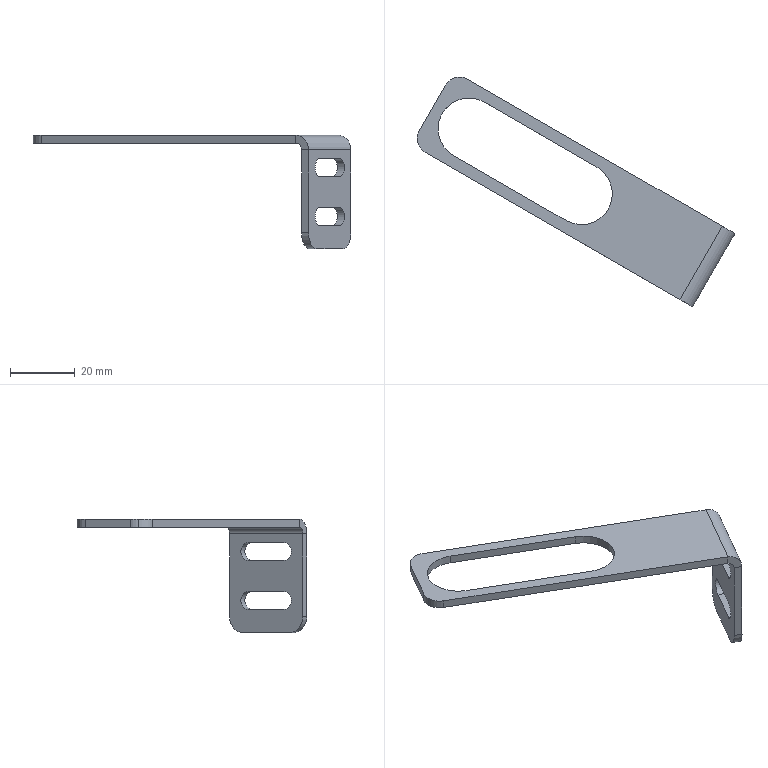Part | STEP file | 1 solid | 34 faces | box 97.772 x 70.687 x 35 mm | volume 5397 mm3 | plane 18 | cylinder 16 | commonest cylinder face diameters 5.5 x6 10 x5 19 x3 4 x1 9 x1